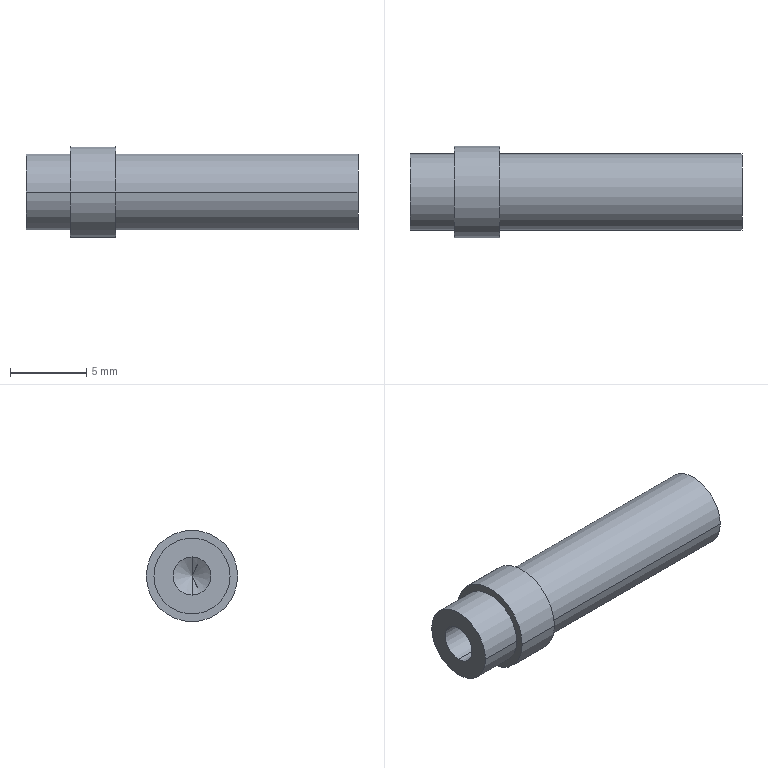Part | SolidWorks | features 3DProfileFeature 1, HoleWzd 1, Revolution 1 | 1 solid | 18 faces | box 21.8 x 6 x 6 mm | volume 372.962 mm3 | cylinder 10 | cone 4 | plane 4 | commonest cylinder face diameters 2.5 x4 5 x4 6 x2
STEP:
#1=CARTESIAN_POINT('',(8.506,-2.5,-1.25));
#2=VERTEX_POINT('',#1);
#3=CARTESIAN_POINT('',(8.506,-2.5,1.25));
#4=VERTEX_POINT('',#3);
#5=CARTESIAN_POINT('',(8.506,-2.5,0.));
#6=DIRECTION('',(-1.,0.,0.));
#7=DIRECTION('',(0.,0.,1.));
#8=AXIS2_PLACEMENT_3D('',#5,#6,#7);
#9=CIRCLE('',#8,1.25);
#10=EDGE_CURVE('',#2,#4,#9,.T.);
#11=ORIENTED_EDGE('',*,*,#10,.F.);
#12=CARTESIAN_POINT('',(0.5057,-2.5,-1.25));
#13=VERTEX_POINT('',#12);
#14=CARTESIAN_POINT('',(0.5057,-2.5,-1.25));
#15=DIRECTION('',(-1.,0.,0.));
#16=VECTOR('',#15,1000.);
#17=LINE('',#14,#16);
#18=EDGE_CURVE('',#2,#13,#17,.T.);
#19=ORIENTED_EDGE('',*,*,#18,.T.);
#20=CARTESIAN_POINT('',(0.5057,-2.5,1.25));
#21=VERTEX_POINT('',#20);
#22=CARTESIAN_POINT('',(0.5057,-2.5,0.));
#23=DIRECTION('',(-1.,0.,0.));
#24=DIRECTION('',(0.,0.,1.));
#25=AXIS2_PLACEMENT_3D('',#22,#23,#24);
#26=CIRCLE('',#25,1.25);
#27=EDGE_CURVE('',#13,#21,#26,.T.);
#28=ORIENTED_EDGE('',*,*,#27,.T.);
#29=CARTESIAN_POINT('',(0.5057,-2.5,1.25));
#30=DIRECTION('',(-1.,0.,0.));
#31=VECTOR('',#30,1000.);
#32=LINE('',#29,#31);
#33=EDGE_CURVE('',#4,#21,#32,.T.);
#34=ORIENTED_EDGE('',*,*,#33,.F.);
#35=EDGE_LOOP('',(#11,#19,#28,#34));
#36=FACE_OUTER_BOUND('',#35,.T.);
#37=CARTESIAN_POINT('',(0.5057,-2.5,0.));
#38=DIRECTION('',(-1.,0.,0.));
#39=DIRECTION('',(0.,0.,1.));
#40=AXIS2_PLACEMENT_3D('',#37,#38,#39);
#41=CYLINDRICAL_SURFACE('',#40,1.25);
#42=ADVANCED_FACE('',(#36),#41,.F.);
#43=CARTESIAN_POINT('',(9.257,-2.5,0.));
#44=VERTEX_POINT('',#43);
#45=CARTESIAN_POINT('',(8.506,-2.5,1.25));
#46=DIRECTION('',(-0.515,0.,0.8572));
#47=VECTOR('',#46,1000.);
#48=LINE('',#45,#47);
#49=EDGE_CURVE('',#44,#4,#48,.T.);
#50=ORIENTED_EDGE('',*,*,#49,.F.);
#51=CARTESIAN_POINT('',(8.506,-2.5,-1.25));
#52=DIRECTION('',(-0.515,0.,-0.8572));
#53=VECTOR('',#52,1000.);
#54=LINE('',#51,#53);
#55=EDGE_CURVE('',#44,#2,#54,.T.);
#56=ORIENTED_EDGE('',*,*,#55,.T.);
#57=ORIENTED_EDGE('',*,*,#10,.T.);
#58=EDGE_LOOP('',(#50,#56,#57));
#59=FACE_OUTER_BOUND('',#58,.T.);
#60=CARTESIAN_POINT('',(8.506,-2.5,0.));
#61=DIRECTION('',(-1.,0.,0.));
#62=DIRECTION('',(0.,0.,1.));
#63=AXIS2_PLACEMENT_3D('',#60,#61,#62);
#64=CONICAL_SURFACE('',#63,1.25,1.03);
#65=ADVANCED_FACE('',(#59),#64,.F.);
#66=CARTESIAN_POINT('',(14.306,-2.5,1.25));
#67=VERTEX_POINT('',#66);
#68=CARTESIAN_POINT('',(14.306,-2.5,-1.25));
#69=VERTEX_POINT('',#68);
#70=CARTESIAN_POINT('',(14.306,-2.5,0.));
#71=DIRECTION('',(1.,0.,0.));
#72=DIRECTION('',(0.,0.,-1.));
#73=AXIS2_PLACEMENT_3D('',#70,#71,#72);
#74=CIRCLE('',#73,1.25);
#75=EDGE_CURVE('',#67,#69,#74,.T.);
#76=ORIENTED_EDGE('',*,*,#75,.F.);
#77=CARTESIAN_POINT('',(22.306,-2.5,1.25));
#78=VERTEX_POINT('',#77);
#79=CARTESIAN_POINT('',(22.306,-2.5,1.25));
#80=DIRECTION('',(1.,0.,0.));
#81=VECTOR('',#80,1000.);
#82=LINE('',#79,#81);
#83=EDGE_CURVE('',#67,#78,#82,.T.);
#84=ORIENTED_EDGE('',*,*,#83,.T.);
#85=CARTESIAN_POINT('',(22.306,-2.5,-1.25));
#86=VERTEX_POINT('',#85);
#87=CARTESIAN_POINT('',(22.306,-2.5,0.));
#88=DIRECTION('',(1.,0.,0.));
#89=DIRECTION('',(0.,0.,-1.));
#90=AXIS2_PLACEMENT_3D('',#87,#88,#89);
#91=CIRCLE('',#90,1.25);
#92=EDGE_CURVE('',#78,#86,#91,.T.);
#93=ORIENTED_EDGE('',*,*,#92,.T.);
#94=CARTESIAN_POINT('',(22.306,-2.5,-1.25));
#95=DIRECTION('',(1.,0.,0.));
#96=VECTOR('',#95,1000.);
#97=LINE('',#94,#96);
#98=EDGE_CURVE('',#69,#86,#97,.T.);
#99=ORIENTED_EDGE('',*,*,#98,.F.);
#100=EDGE_LOOP('',(#76,#84,#93,#99));
#101=FACE_OUTER_BOUND('',#100,.T.);
#102=CARTESIAN_POINT('',(22.306,-2.5,0.));
#103=DIRECTION('',(1.,0.,0.));
#104=DIRECTION('',(0.,0.,-1.));
#105=AXIS2_PLACEMENT_3D('',#102,#103,#104);
#106=CYLINDRICAL_SURFACE('',#105,1.25);
#107=ADVANCED_FACE('',(#101),#106,.F.);
#108=CARTESIAN_POINT('',(13.555,-2.5,0.));
#109=VERTEX_POINT('',#108);
#110=CARTESIAN_POINT('',(14.306,-2.5,-1.25));
#111=DIRECTION('',(0.515,0.,-0.8572));
#112=VECTOR('',#111,1000.);
#113=LINE('',#110,#112);
#114=EDGE_CURVE('',#109,#69,#113,.T.);
#115=ORIENTED_EDGE('',*,*,#114,.F.);
#116=CARTESIAN_POINT('',(14.306,-2.5,1.25));
#117=DIRECTION('',(0.515,0.,0.8572));
#118=VECTOR('',#117,1000.);
#119=LINE('',#116,#118);
#120=EDGE_CURVE('',#109,#67,#119,.T.);
#121=ORIENTED_EDGE('',*,*,#120,.T.);
#122=ORIENTED_EDGE('',*,*,#75,.T.);
#123=EDGE_LOOP('',(#115,#121,#122));
#124=FACE_OUTER_BOUND('',#123,.T.);
#125=CARTESIAN_POINT('',(14.306,-2.5,0.));
#126=DIRECTION('',(1.,0.,0.));
#127=DIRECTION('',(0.,0.,-1.));
#128=AXIS2_PLACEMENT_3D('',#125,#126,#127);
#129=CONICAL_SURFACE('',#128,1.25,1.03);
#130=ADVANCED_FACE('',(#124),#129,.F.);
#131=CARTESIAN_POINT('',(6.406,0.,0.));
#132=VERTEX_POINT('',#131);
#133=CARTESIAN_POINT('',(6.406,-5.,0.));
#134=VERTEX_POINT('',#133);
#135=CARTESIAN_POINT('',(6.406,-2.5,0.));
#136=DIRECTION('',(1.,0.,0.));
#137=DIRECTION('',(0.,1.,0.));
#138=AXIS2_PLACEMENT_3D('',#135,#136,#137);
#139=CIRCLE('',#138,2.5);
#140=EDGE_CURVE('',#132,#134,#139,.T.);
#141=ORIENTED_EDGE('',*,*,#140,.T.);
#142=CARTESIAN_POINT('',(22.306,-5.,0.));
#143=VERTEX_POINT('',#142);
#144=CARTESIAN_POINT('',(22.306,-5.,0.));
#145=DIRECTION('',(1.,0.,0.));
#146=VECTOR('',#145,1000.);
#147=LINE('',#144,#146);
#148=EDGE_CURVE('',#134,#143,#147,.T.);
#149=ORIENTED_EDGE('',*,*,#148,.T.);
#150=CARTESIAN_POINT('',(22.306,0.,0.));
#151=VERTEX_POINT('',#150);
#152=CARTESIAN_POINT('',(22.306,-2.5,0.));
#153=DIRECTION('',(1.,0.,0.));
#154=DIRECTION('',(0.,1.,0.));
#155=AXIS2_PLACEMENT_3D('',#152,#153,#154);
#156=CIRCLE('',#155,2.5);
#157=EDGE_CURVE('',#151,#143,#156,.T.);
#158=ORIENTED_EDGE('',*,*,#157,.F.);
#159=CARTESIAN_POINT('',(22.306,0.,0.));
#160=DIRECTION('',(1.,0.,0.));
#161=VECTOR('',#160,1000.);
#162=LINE('',#159,#161);
#163=EDGE_CURVE('',#132,#151,#162,.T.);
#164=ORIENTED_EDGE('',*,*,#163,.F.);
#165=EDGE_LOOP('',(#141,#149,#158,#164));
#166=FACE_OUTER_BOUND('',#165,.T.);
#167=CARTESIAN_POINT('',(22.306,-2.5,0.));
#168=DIRECTION('',(1.,0.,0.));
#169=DIRECTION('',(0.,1.,0.));
#170=AXIS2_PLACEMENT_3D('',#167,#168,#169);
#171=CYLINDRICAL_SURFACE('',#170,2.5);
#172=ADVANCED_FACE('',(#166),#171,.T.);
#173=CARTESIAN_POINT('',(3.406,0.5,0.));
#174=VERTEX_POINT('',#173);
#175=CARTESIAN_POINT('',(3.406,-5.5,0.));
#176=VERTEX_POINT('',#175);
#177=CARTESIAN_POINT('',(3.406,-2.5,0.));
#178=DIRECTION('',(1.,0.,0.));
#179=DIRECTION('',(0.,1.,0.));
#180=AXIS2_PLACEMENT_3D('',#177,#178,#179);
#181=CIRCLE('',#180,3.);
#182=EDGE_CURVE('',#174,#176,#181,.T.);
#183=ORIENTED_EDGE('',*,*,#182,.T.);
#184=CARTESIAN_POINT('',(6.406,-5.5,0.));
#185=VERTEX_POINT('',#184);
#186=CARTESIAN_POINT('',(22.306,-5.5,0.));
#187=DIRECTION('',(1.,0.,0.));
#188=VECTOR('',#187,1000.);
#189=LINE('',#186,#188);
#190=EDGE_CURVE('',#176,#185,#189,.T.);
#191=ORIENTED_EDGE('',*,*,#190,.T.);
#192=CARTESIAN_POINT('',(6.406,0.5,0.));
#193=VERTEX_POINT('',#192);
#194=CARTESIAN_POINT('',(6.406,-2.5,0.));
#195=DIRECTION('',(1.,0.,0.));
#196=DIRECTION('',(0.,1.,0.));
#197=AXIS2_PLACEMENT_3D('',#194,#195,#196);
#198=CIRCLE('',#197,3.);
#199=EDGE_CURVE('',#193,#185,#198,.T.);
#200=ORIENTED_EDGE('',*,*,#199,.F.);
#201=CARTESIAN_POINT('',(22.306,0.5,0.));
#202=DIRECTION('',(1.,0.,0.));
#203=VECTOR('',#202,1000.);
#204=LINE('',#201,#203);
#205=EDGE_CURVE('',#174,#193,#204,.T.);
#206=ORIENTED_EDGE('',*,*,#205,.F.);
#207=EDGE_LOOP('',(#183,#191,#200,#206));
#208=FACE_OUTER_BOUND('',#207,.T.);
#209=CARTESIAN_POINT('',(22.306,-2.5,0.));
#210=DIRECTION('',(1.,0.,0.));
#211=DIRECTION('',(0.,1.,0.));
#212=AXIS2_PLACEMENT_3D('',#209,#210,#211);
#213=CYLINDRICAL_SURFACE('',#212,3.);
#214=ADVANCED_FACE('',(#208),#213,.T.);
#215=CARTESIAN_POINT('',(0.5057,0.,0.));
#216=VERTEX_POINT('',#215);
#217=CARTESIAN_POINT('',(0.5057,-5.,0.));
#218=VERTEX_POINT('',#217);
#219=CARTESIAN_POINT('',(0.5057,-2.5,0.));
#220=DIRECTION('',(1.,0.,0.));
#221=DIRECTION('',(0.,1.,0.));
#222=AXIS2_PLACEMENT_3D('',#219,#220,#221);
#223=CIRCLE('',#222,2.5);
#224=EDGE_CURVE('',#216,#218,#223,.T.);
#225=ORIENTED_EDGE('',*,*,#224,.T.);
#226=CARTESIAN_POINT('',(3.406,-5.,0.));
#227=VERTEX_POINT('',#226);
#228=CARTESIAN_POINT('',(22.306,-5.,0.));
#229=DIRECTION('',(1.,0.,0.));
#230=VECTOR('',#229,1000.);
#231=LINE('',#228,#230);
#232=EDGE_CURVE('',#218,#227,#231,.T.);
#233=ORIENTED_EDGE('',*,*,#232,.T.);
#234=CARTESIAN_POINT('',(3.406,0.,0.));
#235=VERTEX_POINT('',#234);
#236=CARTESIAN_POINT('',(3.406,-2.5,0.));
#237=DIRECTION('',(1.,0.,0.));
#238=DIRECTION('',(0.,1.,0.));
#239=AXIS2_PLACEMENT_3D('',#236,#237,#238);
#240=CIRCLE('',#239,2.5);
#241=EDGE_CURVE('',#235,#227,#240,.T.);
#242=ORIENTED_EDGE('',*,*,#241,.F.);
#243=CARTESIAN_POINT('',(22.306,0.,0.));
#244=DIRECTION('',(1.,0.,0.));
#245=VECTOR('',#244,1000.);
#246=LINE('',#243,#245);
#247=EDGE_CURVE('',#216,#235,#246,.T.);
#248=ORIENTED_EDGE('',*,*,#247,.F.);
#249=EDGE_LOOP('',(#225,#233,#242,#248));
#250=FACE_OUTER_BOUND('',#249,.T.);
#251=CARTESIAN_POINT('',(22.306,-2.5,0.));
#252=DIRECTION('',(1.,0.,0.));
#253=DIRECTION('',(0.,1.,0.));
#254=AXIS2_PLACEMENT_3D('',#251,#252,#253);
#255=CYLINDRICAL_SURFACE('',#254,2.5);
#256=ADVANCED_FACE('',(#250),#255,.T.);
#257=CARTESIAN_POINT('',(0.5057,-2.5,0.));
#258=DIRECTION('',(-1.,0.,0.));
#259=DIRECTION('',(0.,0.,1.));
#260=AXIS2_PLACEMENT_3D('',#257,#258,#259);
#261=CIRCLE('',#260,1.25);
#262=EDGE_CURVE('',#21,#13,#261,.T.);
#263=ORIENTED_EDGE('',*,*,#262,.F.);
#264=ORIENTED_EDGE('',*,*,#27,.F.);
#265=EDGE_LOOP('',(#263,#264));
#266=FACE_BOUND('',#265,.T.);
#267=ORIENTED_EDGE('',*,*,#224,.F.);
#268=CARTESIAN_POINT('',(0.5057,-2.5,0.));
#269=DIRECTION('',(1.,0.,0.));
#270=DIRECTION('',(0.,1.,0.));
#271=AXIS2_PLACEMENT_3D('',#268,#269,#270);
#272=CIRCLE('',#271,2.5);
#273=EDGE_CURVE('',#218,#216,#272,.T.);
#274=ORIENTED_EDGE('',*,*,#273,.F.);
#275=EDGE_LOOP('',(#267,#274));
#276=FACE_OUTER_BOUND('',#275,.T.);
#277=CARTESIAN_POINT('',(0.5057,-2.5,0.));
#278=DIRECTION('',(-1.,0.,0.));
#279=DIRECTION('',(0.,-1.,0.));
#280=AXIS2_PLACEMENT_3D('',#277,#278,#279);
#281=PLANE('',#280);
#282=ADVANCED_FACE('',(#266,#276),#281,.T.);
#283=ORIENTED_EDGE('',*,*,#232,.F.);
#284=ORIENTED_EDGE('',*,*,#273,.T.);
#285=ORIENTED_EDGE('',*,*,#247,.T.);
#286=CARTESIAN_POINT('',(3.406,-2.5,0.));
#287=DIRECTION('',(1.,0.,0.));
#288=DIRECTION('',(0.,1.,0.));
#289=AXIS2_PLACEMENT_3D('',#286,#287,#288);
#290=CIRCLE('',#289,2.5);
#291=EDGE_CURVE('',#227,#235,#290,.T.);
#292=ORIENTED_EDGE('',*,*,#291,.F.);
#293=EDGE_LOOP('',(#283,#284,#285,#292));
#294=FACE_OUTER_BOUND('',#293,.T.);
#295=CARTESIAN_POINT('',(22.306,-2.5,0.));
#296=DIRECTION('',(1.,0.,0.));
#297=DIRECTION('',(0.,1.,0.));
#298=AXIS2_PLACEMENT_3D('',#295,#296,#297);
#299=CYLINDRICAL_SURFACE('',#298,2.5);
#300=ADVANCED_FACE('',(#294),#299,.T.);
#301=ORIENTED_EDGE('',*,*,#241,.T.);
#302=ORIENTED_EDGE('',*,*,#291,.T.);
#303=EDGE_LOOP('',(#301,#302));
#304=FACE_BOUND('',#303,.T.);
#305=ORIENTED_EDGE('',*,*,#182,.F.);
#306=CARTESIAN_POINT('',(3.406,-2.5,0.));
#307=DIRECTION('',(1.,0.,0.));
#308=DIRECTION('',(0.,1.,0.));
#309=AXIS2_PLACEMENT_3D('',#306,#307,#308);
#310=CIRCLE('',#309,3.);
#311=EDGE_CURVE('',#176,#174,#310,.T.);
#312=ORIENTED_EDGE('',*,*,#311,.F.);
#313=EDGE_LOOP('',(#305,#312));
#314=FACE_OUTER_BOUND('',#313,.T.);
#315=CARTESIAN_POINT('',(3.406,0.,0.));
#316=DIRECTION('',(-1.,0.,0.));
#317=DIRECTION('',(0.,-1.,0.));
#318=AXIS2_PLACEMENT_3D('',#315,#316,#317);
#319=PLANE('',#318);
#320=ADVANCED_FACE('',(#304,#314),#319,.T.);
#321=ORIENTED_EDGE('',*,*,#190,.F.);
#322=ORIENTED_EDGE('',*,*,#311,.T.);
#323=ORIENTED_EDGE('',*,*,#205,.T.);
#324=CARTESIAN_POINT('',(6.406,-2.5,0.));
#325=DIRECTION('',(1.,0.,0.));
#326=DIRECTION('',(0.,1.,0.));
#327=AXIS2_PLACEMENT_3D('',#324,#325,#326);
#328=CIRCLE('',#327,3.);
#329=EDGE_CURVE('',#185,#193,#328,.T.);
#330=ORIENTED_EDGE('',*,*,#329,.F.);
#331=EDGE_LOOP('',(#321,#322,#323,#330));
#332=FACE_OUTER_BOUND('',#331,.T.);
#333=CARTESIAN_POINT('',(22.306,-2.5,0.));
#334=DIRECTION('',(1.,0.,0.));
#335=DIRECTION('',(0.,1.,0.));
#336=AXIS2_PLACEMENT_3D('',#333,#334,#335);
#337=CYLINDRICAL_SURFACE('',#336,3.);
#338=ADVANCED_FACE('',(#332),#337,.T.);
#339=ORIENTED_EDGE('',*,*,#199,.T.);
#340=ORIENTED_EDGE('',*,*,#329,.T.);
#341=EDGE_LOOP('',(#339,#340));
#342=FACE_OUTER_BOUND('',#341,.T.);
#343=ORIENTED_EDGE('',*,*,#140,.F.);
#344=CARTESIAN_POINT('',(6.406,-2.5,0.));
#345=DIRECTION('',(1.,0.,0.));
#346=DIRECTION('',(0.,1.,0.));
#347=AXIS2_PLACEMENT_3D('',#344,#345,#346);
#348=CIRCLE('',#347,2.5);
#349=EDGE_CURVE('',#134,#132,#348,.T.);
#350=ORIENTED_EDGE('',*,*,#349,.F.);
#351=EDGE_LOOP('',(#343,#350));
#352=FACE_BOUND('',#351,.T.);
#353=CARTESIAN_POINT('',(6.406,0.5,0.));
#354=DIRECTION('',(1.,0.,0.));
#355=DIRECTION('',(0.,1.,0.));
#356=AXIS2_PLACEMENT_3D('',#353,#354,#355);
#357=PLANE('',#356);
#358=ADVANCED_FACE('',(#342,#352),#357,.T.);
#359=ORIENTED_EDGE('',*,*,#148,.F.);
#360=ORIENTED_EDGE('',*,*,#349,.T.);
#361=ORIENTED_EDGE('',*,*,#163,.T.);
#362=CARTESIAN_POINT('',(22.306,-2.5,0.));
#363=DIRECTION('',(1.,0.,0.));
#364=DIRECTION('',(0.,1.,0.));
#365=AXIS2_PLACEMENT_3D('',#362,#363,#364);
#366=CIRCLE('',#365,2.5);
#367=EDGE_CURVE('',#143,#151,#366,.T.);
#368=ORIENTED_EDGE('',*,*,#367,.F.);
#369=EDGE_LOOP('',(#359,#360,#361,#368));
#370=FACE_OUTER_BOUND('',#369,.T.);
#371=CARTESIAN_POINT('',(22.306,-2.5,0.));
#372=DIRECTION('',(1.,0.,0.));
#373=DIRECTION('',(0.,1.,0.));
#374=AXIS2_PLACEMENT_3D('',#371,#372,#373);
#375=CYLINDRICAL_SURFACE('',#374,2.5);
#376=ADVANCED_FACE('',(#370),#375,.T.);
#377=CARTESIAN_POINT('',(22.306,-2.5,0.));
#378=DIRECTION('',(1.,0.,0.));
#379=DIRECTION('',(0.,0.,-1.));
#380=AXIS2_PLACEMENT_3D('',#377,#378,#379);
#381=CIRCLE('',#380,1.25);
#382=EDGE_CURVE('',#86,#78,#381,.T.);
#383=ORIENTED_EDGE('',*,*,#382,.F.);
#384=ORIENTED_EDGE('',*,*,#92,.F.);
#385=EDGE_LOOP('',(#383,#384));
#386=FACE_BOUND('',#385,.T.);
#387=ORIENTED_EDGE('',*,*,#157,.T.);
#388=ORIENTED_EDGE('',*,*,#367,.T.);
#389=EDGE_LOOP('',(#387,#388));
#390=FACE_OUTER_BOUND('',#389,.T.);
#391=CARTESIAN_POINT('',(22.306,0.,0.));
#392=DIRECTION('',(1.,0.,0.));
#393=DIRECTION('',(0.,1.,0.));
#394=AXIS2_PLACEMENT_3D('',#391,#392,#393);
#395=PLANE('',#394);
#396=ADVANCED_FACE('',(#386,#390),#395,.T.);
#397=ORIENTED_EDGE('',*,*,#120,.F.);
#398=ORIENTED_EDGE('',*,*,#114,.T.);
#399=CARTESIAN_POINT('',(14.306,-2.5,0.));
#400=DIRECTION('',(1.,0.,0.));
#401=DIRECTION('',(0.,0.,-1.));
#402=AXIS2_PLACEMENT_3D('',#399,#400,#401);
#403=CIRCLE('',#402,1.25);
#404=EDGE_CURVE('',#69,#67,#403,.T.);
#405=ORIENTED_EDGE('',*,*,#404,.T.);
#406=EDGE_LOOP('',(#397,#398,#405));
#407=FACE_OUTER_BOUND('',#406,.T.);
#408=CARTESIAN_POINT('',(14.306,-2.5,0.));
#409=DIRECTION('',(1.,0.,0.));
#410=DIRECTION('',(0.,0.,-1.));
#411=AXIS2_PLACEMENT_3D('',#408,#409,#410);
#412=CONICAL_SURFACE('',#411,1.25,1.03);
#413=ADVANCED_FACE('',(#407),#412,.F.);
#414=ORIENTED_EDGE('',*,*,#83,.F.);
#415=ORIENTED_EDGE('',*,*,#404,.F.);
#416=ORIENTED_EDGE('',*,*,#98,.T.);
#417=ORIENTED_EDGE('',*,*,#382,.T.);
#418=EDGE_LOOP('',(#414,#415,#416,#417));
#419=FACE_OUTER_BOUND('',#418,.T.);
#420=CARTESIAN_POINT('',(22.306,-2.5,0.));
#421=DIRECTION('',(1.,0.,0.));
#422=DIRECTION('',(0.,0.,-1.));
#423=AXIS2_PLACEMENT_3D('',#420,#421,#422);
#424=CYLINDRICAL_SURFACE('',#423,1.25);
#425=ADVANCED_FACE('',(#419),#424,.F.);
#426=ORIENTED_EDGE('',*,*,#55,.F.);
#427=ORIENTED_EDGE('',*,*,#49,.T.);
#428=CARTESIAN_POINT('',(8.506,-2.5,0.));
#429=DIRECTION('',(-1.,0.,0.));
#430=DIRECTION('',(0.,0.,1.));
#431=AXIS2_PLACEMENT_3D('',#428,#429,#430);
#432=CIRCLE('',#431,1.25);
#433=EDGE_CURVE('',#4,#2,#432,.T.);
#434=ORIENTED_EDGE('',*,*,#433,.T.);
#435=EDGE_LOOP('',(#426,#427,#434));
#436=FACE_OUTER_BOUND('',#435,.T.);
#437=CARTESIAN_POINT('',(8.506,-2.5,0.));
#438=DIRECTION('',(-1.,0.,0.));
#439=DIRECTION('',(0.,0.,1.));
#440=AXIS2_PLACEMENT_3D('',#437,#438,#439);
#441=CONICAL_SURFACE('',#440,1.25,1.03);
#442=ADVANCED_FACE('',(#436),#441,.F.);
#443=ORIENTED_EDGE('',*,*,#18,.F.);
#444=ORIENTED_EDGE('',*,*,#433,.F.);
#445=ORIENTED_EDGE('',*,*,#33,.T.);
#446=ORIENTED_EDGE('',*,*,#262,.T.);
#447=EDGE_LOOP('',(#443,#444,#445,#446));
#448=FACE_OUTER_BOUND('',#447,.T.);
#449=CARTESIAN_POINT('',(0.5057,-2.5,0.));
#450=DIRECTION('',(-1.,0.,0.));
#451=DIRECTION('',(0.,0.,1.));
#452=AXIS2_PLACEMENT_3D('',#449,#450,#451);
#453=CYLINDRICAL_SURFACE('',#452,1.25);
#454=ADVANCED_FACE('',(#448),#453,.F.);
#455=CLOSED_SHELL('',(#42,#65,#107,#130,#172,#214,#256,#282,#300,#320,#338,#358,#376,#396,#413,#425,#442,#454));
#456=MANIFOLD_SOLID_BREP('',#455);
#457=CARTESIAN_POINT('',(0.,0.,0.));
#458=DIRECTION('',(0.,0.,1.));
#459=DIRECTION('',(1.,0.,0.));
#460=AXIS2_PLACEMENT_3D('',#457,#458,#459);
#461=(LENGTH_UNIT()NAMED_UNIT(*)SI_UNIT(.MILLI.,.METRE.));
#462=UNCERTAINTY_MEASURE_WITH_UNIT(LENGTH_MEASURE(0.00001),#461,'','');
#463=(NAMED_UNIT(*)PLANE_ANGLE_UNIT()SI_UNIT($,.RADIAN.));
#464=(NAMED_UNIT(*)SI_UNIT($,.STERADIAN.)SOLID_ANGLE_UNIT());
#465=(GEOMETRIC_REPRESENTATION_CONTEXT(3)GLOBAL_UNCERTAINTY_ASSIGNED_CONTEXT((#462))GLOBAL_UNIT_ASSIGNED_CONTEXT((#461,#463,#464))REPRESENTATION_CONTEXT('',''));
#466=ADVANCED_BREP_SHAPE_REPRESENTATION('',(#456,#460),#465);